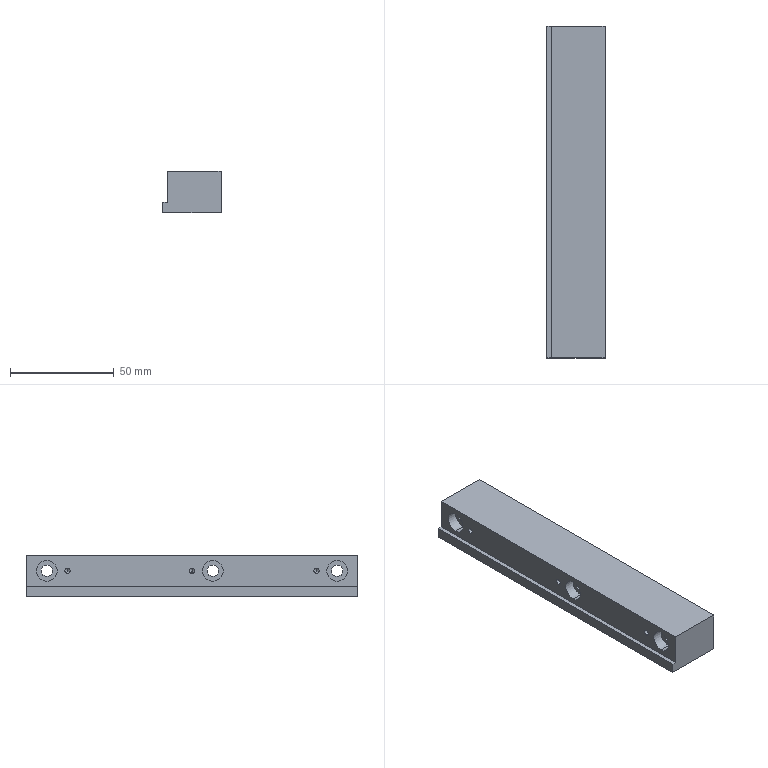Part | SolidWorks | features LPattern 3, HoleWzd 2, Extrusion 1, ICE 1 | 1 solid | 35 faces | box 28 x 160 x 20 mm | volume 82011 mm3 | cylinder 18 | plane 11 | cone 6 | commonest cylinder face diameters 2.5 x6 5.5 x6 10 x6
STEP:
#1=CARTESIAN_POINT('',(7.,-10.,-2.5));
#2=VERTEX_POINT('',#1);
#3=CARTESIAN_POINT('',(7.,-10.,7.5));
#4=VERTEX_POINT('',#3);
#5=CARTESIAN_POINT('',(7.,-10.,2.5));
#6=DIRECTION('',(-1.,0.,0.));
#7=DIRECTION('',(0.,0.,1.));
#8=AXIS2_PLACEMENT_3D('',#5,#6,#7);
#9=CIRCLE('',#8,5.);
#10=EDGE_CURVE('',#2,#4,#9,.T.);
#11=ORIENTED_EDGE('',*,*,#10,.F.);
#12=CARTESIAN_POINT('',(2.,-10.,-2.5));
#13=VERTEX_POINT('',#12);
#14=CARTESIAN_POINT('',(2.,-10.,-2.5));
#15=DIRECTION('',(-1.,0.,0.));
#16=VECTOR('',#15,1000.);
#17=LINE('',#14,#16);
#18=EDGE_CURVE('',#2,#13,#17,.T.);
#19=ORIENTED_EDGE('',*,*,#18,.T.);
#20=CARTESIAN_POINT('',(2.,-10.,7.5));
#21=VERTEX_POINT('',#20);
#22=CARTESIAN_POINT('',(2.,-10.,2.5));
#23=DIRECTION('',(-1.,0.,0.));
#24=DIRECTION('',(0.,0.,1.));
#25=AXIS2_PLACEMENT_3D('',#22,#23,#24);
#26=CIRCLE('',#25,5.);
#27=EDGE_CURVE('',#13,#21,#26,.T.);
#28=ORIENTED_EDGE('',*,*,#27,.T.);
#29=CARTESIAN_POINT('',(2.,-10.,7.5));
#30=DIRECTION('',(-1.,0.,0.));
#31=VECTOR('',#30,1000.);
#32=LINE('',#29,#31);
#33=EDGE_CURVE('',#4,#21,#32,.T.);
#34=ORIENTED_EDGE('',*,*,#33,.F.);
#35=EDGE_LOOP('',(#11,#19,#28,#34));
#36=FACE_OUTER_BOUND('',#35,.T.);
#37=CARTESIAN_POINT('',(2.,-10.,2.5));
#38=DIRECTION('',(-1.,0.,0.));
#39=DIRECTION('',(0.,0.,1.));
#40=AXIS2_PLACEMENT_3D('',#37,#38,#39);
#41=CYLINDRICAL_SURFACE('',#40,5.);
#42=ADVANCED_FACE('',(#36),#41,.F.);
#43=CARTESIAN_POINT('',(28.,-10.,-0.25));
#44=VERTEX_POINT('',#43);
#45=CARTESIAN_POINT('',(28.,-10.,5.25));
#46=VERTEX_POINT('',#45);
#47=CARTESIAN_POINT('',(28.,-10.,2.5));
#48=DIRECTION('',(-1.,0.,0.));
#49=DIRECTION('',(0.,0.,1.));
#50=AXIS2_PLACEMENT_3D('',#47,#48,#49);
#51=CIRCLE('',#50,2.75);
#52=EDGE_CURVE('',#44,#46,#51,.T.);
#53=ORIENTED_EDGE('',*,*,#52,.F.);
#54=CARTESIAN_POINT('',(7.,-10.,-0.25));
#55=VERTEX_POINT('',#54);
#56=CARTESIAN_POINT('',(2.,-10.,-0.25));
#57=DIRECTION('',(-1.,0.,0.));
#58=VECTOR('',#57,1000.);
#59=LINE('',#56,#58);
#60=EDGE_CURVE('',#44,#55,#59,.T.);
#61=ORIENTED_EDGE('',*,*,#60,.T.);
#62=CARTESIAN_POINT('',(7.,-10.,5.25));
#63=VERTEX_POINT('',#62);
#64=CARTESIAN_POINT('',(7.,-10.,2.5));
#65=DIRECTION('',(-1.,0.,0.));
#66=DIRECTION('',(0.,0.,1.));
#67=AXIS2_PLACEMENT_3D('',#64,#65,#66);
#68=CIRCLE('',#67,2.75);
#69=EDGE_CURVE('',#55,#63,#68,.T.);
#70=ORIENTED_EDGE('',*,*,#69,.T.);
#71=CARTESIAN_POINT('',(2.,-10.,5.25));
#72=DIRECTION('',(-1.,0.,0.));
#73=VECTOR('',#72,1000.);
#74=LINE('',#71,#73);
#75=EDGE_CURVE('',#46,#63,#74,.T.);
#76=ORIENTED_EDGE('',*,*,#75,.F.);
#77=EDGE_LOOP('',(#53,#61,#70,#76));
#78=FACE_OUTER_BOUND('',#77,.T.);
#79=CARTESIAN_POINT('',(2.,-10.,2.5));
#80=DIRECTION('',(-1.,0.,0.));
#81=DIRECTION('',(0.,0.,1.));
#82=AXIS2_PLACEMENT_3D('',#79,#80,#81);
#83=CYLINDRICAL_SURFACE('',#82,2.75);
#84=ADVANCED_FACE('',(#78),#83,.F.);
#85=CARTESIAN_POINT('',(7.,70.,-2.5));
#86=VERTEX_POINT('',#85);
#87=CARTESIAN_POINT('',(7.,70.,7.5));
#88=VERTEX_POINT('',#87);
#89=CARTESIAN_POINT('',(7.,70.,2.5));
#90=DIRECTION('',(-1.,0.,0.));
#91=DIRECTION('',(0.,0.,1.));
#92=AXIS2_PLACEMENT_3D('',#89,#90,#91);
#93=CIRCLE('',#92,5.);
#94=EDGE_CURVE('',#86,#88,#93,.T.);
#95=ORIENTED_EDGE('',*,*,#94,.F.);
#96=CARTESIAN_POINT('',(2.,70.,-2.5));
#97=VERTEX_POINT('',#96);
#98=CARTESIAN_POINT('',(2.,70.,-2.5));
#99=DIRECTION('',(-1.,0.,0.));
#100=VECTOR('',#99,1000.);
#101=LINE('',#98,#100);
#102=EDGE_CURVE('',#86,#97,#101,.T.);
#103=ORIENTED_EDGE('',*,*,#102,.T.);
#104=CARTESIAN_POINT('',(2.,70.,7.5));
#105=VERTEX_POINT('',#104);
#106=CARTESIAN_POINT('',(2.,70.,2.5));
#107=DIRECTION('',(-1.,0.,0.));
#108=DIRECTION('',(0.,0.,1.));
#109=AXIS2_PLACEMENT_3D('',#106,#107,#108);
#110=CIRCLE('',#109,5.);
#111=EDGE_CURVE('',#97,#105,#110,.T.);
#112=ORIENTED_EDGE('',*,*,#111,.T.);
#113=CARTESIAN_POINT('',(2.,70.,7.5));
#114=DIRECTION('',(-1.,0.,0.));
#115=VECTOR('',#114,1000.);
#116=LINE('',#113,#115);
#117=EDGE_CURVE('',#88,#105,#116,.T.);
#118=ORIENTED_EDGE('',*,*,#117,.F.);
#119=EDGE_LOOP('',(#95,#103,#112,#118));
#120=FACE_OUTER_BOUND('',#119,.T.);
#121=CARTESIAN_POINT('',(2.,70.,2.5));
#122=DIRECTION('',(-1.,0.,0.));
#123=DIRECTION('',(0.,0.,1.));
#124=AXIS2_PLACEMENT_3D('',#121,#122,#123);
#125=CYLINDRICAL_SURFACE('',#124,5.);
#126=ADVANCED_FACE('',(#120),#125,.F.);
#127=CARTESIAN_POINT('',(28.,70.,-0.25));
#128=VERTEX_POINT('',#127);
#129=CARTESIAN_POINT('',(28.,70.,5.25));
#130=VERTEX_POINT('',#129);
#131=CARTESIAN_POINT('',(28.,70.,2.5));
#132=DIRECTION('',(-1.,0.,0.));
#133=DIRECTION('',(0.,0.,1.));
#134=AXIS2_PLACEMENT_3D('',#131,#132,#133);
#135=CIRCLE('',#134,2.75);
#136=EDGE_CURVE('',#128,#130,#135,.T.);
#137=ORIENTED_EDGE('',*,*,#136,.F.);
#138=CARTESIAN_POINT('',(7.,70.,-0.25));
#139=VERTEX_POINT('',#138);
#140=CARTESIAN_POINT('',(2.,70.,-0.25));
#141=DIRECTION('',(-1.,0.,0.));
#142=VECTOR('',#141,1000.);
#143=LINE('',#140,#142);
#144=EDGE_CURVE('',#128,#139,#143,.T.);
#145=ORIENTED_EDGE('',*,*,#144,.T.);
#146=CARTESIAN_POINT('',(7.,70.,5.25));
#147=VERTEX_POINT('',#146);
#148=CARTESIAN_POINT('',(7.,70.,2.5));
#149=DIRECTION('',(-1.,0.,0.));
#150=DIRECTION('',(0.,0.,1.));
#151=AXIS2_PLACEMENT_3D('',#148,#149,#150);
#152=CIRCLE('',#151,2.75);
#153=EDGE_CURVE('',#139,#147,#152,.T.);
#154=ORIENTED_EDGE('',*,*,#153,.T.);
#155=CARTESIAN_POINT('',(2.,70.,5.25));
#156=DIRECTION('',(-1.,0.,0.));
#157=VECTOR('',#156,1000.);
#158=LINE('',#155,#157);
#159=EDGE_CURVE('',#130,#147,#158,.T.);
#160=ORIENTED_EDGE('',*,*,#159,.F.);
#161=EDGE_LOOP('',(#137,#145,#154,#160));
#162=FACE_OUTER_BOUND('',#161,.T.);
#163=CARTESIAN_POINT('',(2.,70.,2.5));
#164=DIRECTION('',(-1.,0.,0.));
#165=DIRECTION('',(0.,0.,1.));
#166=AXIS2_PLACEMENT_3D('',#163,#164,#165);
#167=CYLINDRICAL_SURFACE('',#166,2.75);
#168=ADVANCED_FACE('',(#162),#167,.F.);
#169=CARTESIAN_POINT('',(7.,-70.,-2.5));
#170=VERTEX_POINT('',#169);
#171=CARTESIAN_POINT('',(7.,-70.,7.5));
#172=VERTEX_POINT('',#171);
#173=CARTESIAN_POINT('',(7.,-70.,2.5));
#174=DIRECTION('',(-1.,0.,0.));
#175=DIRECTION('',(0.,0.,1.));
#176=AXIS2_PLACEMENT_3D('',#173,#174,#175);
#177=CIRCLE('',#176,5.);
#178=EDGE_CURVE('',#170,#172,#177,.T.);
#179=ORIENTED_EDGE('',*,*,#178,.F.);
#180=CARTESIAN_POINT('',(2.,-70.,-2.5));
#181=VERTEX_POINT('',#180);
#182=CARTESIAN_POINT('',(2.,-70.,-2.5));
#183=DIRECTION('',(-1.,0.,0.));
#184=VECTOR('',#183,1000.);
#185=LINE('',#182,#184);
#186=EDGE_CURVE('',#170,#181,#185,.T.);
#187=ORIENTED_EDGE('',*,*,#186,.T.);
#188=CARTESIAN_POINT('',(2.,-70.,7.5));
#189=VERTEX_POINT('',#188);
#190=CARTESIAN_POINT('',(2.,-70.,2.5));
#191=DIRECTION('',(-1.,0.,0.));
#192=DIRECTION('',(0.,0.,1.));
#193=AXIS2_PLACEMENT_3D('',#190,#191,#192);
#194=CIRCLE('',#193,5.);
#195=EDGE_CURVE('',#181,#189,#194,.T.);
#196=ORIENTED_EDGE('',*,*,#195,.T.);
#197=CARTESIAN_POINT('',(2.,-70.,7.5));
#198=DIRECTION('',(-1.,0.,0.));
#199=VECTOR('',#198,1000.);
#200=LINE('',#197,#199);
#201=EDGE_CURVE('',#172,#189,#200,.T.);
#202=ORIENTED_EDGE('',*,*,#201,.F.);
#203=EDGE_LOOP('',(#179,#187,#196,#202));
#204=FACE_OUTER_BOUND('',#203,.T.);
#205=CARTESIAN_POINT('',(2.,-70.,2.5));
#206=DIRECTION('',(-1.,0.,0.));
#207=DIRECTION('',(0.,0.,1.));
#208=AXIS2_PLACEMENT_3D('',#205,#206,#207);
#209=CYLINDRICAL_SURFACE('',#208,5.);
#210=ADVANCED_FACE('',(#204),#209,.F.);
#211=CARTESIAN_POINT('',(28.,-70.,-0.25));
#212=VERTEX_POINT('',#211);
#213=CARTESIAN_POINT('',(28.,-70.,5.25));
#214=VERTEX_POINT('',#213);
#215=CARTESIAN_POINT('',(28.,-70.,2.5));
#216=DIRECTION('',(-1.,0.,0.));
#217=DIRECTION('',(0.,0.,1.));
#218=AXIS2_PLACEMENT_3D('',#215,#216,#217);
#219=CIRCLE('',#218,2.75);
#220=EDGE_CURVE('',#212,#214,#219,.T.);
#221=ORIENTED_EDGE('',*,*,#220,.F.);
#222=CARTESIAN_POINT('',(7.,-70.,-0.25));
#223=VERTEX_POINT('',#222);
#224=CARTESIAN_POINT('',(2.,-70.,-0.25));
#225=DIRECTION('',(-1.,0.,0.));
#226=VECTOR('',#225,1000.);
#227=LINE('',#224,#226);
#228=EDGE_CURVE('',#212,#223,#227,.T.);
#229=ORIENTED_EDGE('',*,*,#228,.T.);
#230=CARTESIAN_POINT('',(7.,-70.,5.25));
#231=VERTEX_POINT('',#230);
#232=CARTESIAN_POINT('',(7.,-70.,2.5));
#233=DIRECTION('',(-1.,0.,0.));
#234=DIRECTION('',(0.,0.,1.));
#235=AXIS2_PLACEMENT_3D('',#232,#233,#234);
#236=CIRCLE('',#235,2.75);
#237=EDGE_CURVE('',#223,#231,#236,.T.);
#238=ORIENTED_EDGE('',*,*,#237,.T.);
#239=CARTESIAN_POINT('',(2.,-70.,5.25));
#240=DIRECTION('',(-1.,0.,0.));
#241=VECTOR('',#240,1000.);
#242=LINE('',#239,#241);
#243=EDGE_CURVE('',#214,#231,#242,.T.);
#244=ORIENTED_EDGE('',*,*,#243,.F.);
#245=EDGE_LOOP('',(#221,#229,#238,#244));
#246=FACE_OUTER_BOUND('',#245,.T.);
#247=CARTESIAN_POINT('',(2.,-70.,2.5));
#248=DIRECTION('',(-1.,0.,0.));
#249=DIRECTION('',(0.,0.,1.));
#250=AXIS2_PLACEMENT_3D('',#247,#248,#249);
#251=CYLINDRICAL_SURFACE('',#250,2.75);
#252=ADVANCED_FACE('',(#246),#251,.F.);
#253=CARTESIAN_POINT('',(10.251,60.,2.5));
#254=VERTEX_POINT('',#253);
#255=CARTESIAN_POINT('',(9.5,60.,3.75));
#256=VERTEX_POINT('',#255);
#257=CARTESIAN_POINT('',(9.5,60.,3.75));
#258=DIRECTION('',(-0.515,0.,0.8572));
#259=VECTOR('',#258,1000.);
#260=LINE('',#257,#259);
#261=EDGE_CURVE('',#254,#256,#260,.T.);
#262=ORIENTED_EDGE('',*,*,#261,.F.);
#263=CARTESIAN_POINT('',(9.5,60.,1.25));
#264=VERTEX_POINT('',#263);
#265=CARTESIAN_POINT('',(9.5,60.,1.25));
#266=DIRECTION('',(-0.515,0.,-0.8572));
#267=VECTOR('',#266,1000.);
#268=LINE('',#265,#267);
#269=EDGE_CURVE('',#254,#264,#268,.T.);
#270=ORIENTED_EDGE('',*,*,#269,.T.);
#271=CARTESIAN_POINT('',(9.5,60.,2.5));
#272=DIRECTION('',(-1.,0.,0.));
#273=DIRECTION('',(0.,0.,1.));
#274=AXIS2_PLACEMENT_3D('',#271,#272,#273);
#275=CIRCLE('',#274,1.25);
#276=EDGE_CURVE('',#264,#256,#275,.T.);
#277=ORIENTED_EDGE('',*,*,#276,.T.);
#278=EDGE_LOOP('',(#262,#270,#277));
#279=FACE_OUTER_BOUND('',#278,.T.);
#280=CARTESIAN_POINT('',(9.5,60.,2.5));
#281=DIRECTION('',(-1.,0.,0.));
#282=DIRECTION('',(0.,0.,1.));
#283=AXIS2_PLACEMENT_3D('',#280,#281,#282);
#284=CONICAL_SURFACE('',#283,1.25,1.03);
#285=ADVANCED_FACE('',(#279),#284,.F.);
#286=ORIENTED_EDGE('',*,*,#276,.F.);
#287=CARTESIAN_POINT('',(2.,60.,1.25));
#288=VERTEX_POINT('',#287);
#289=CARTESIAN_POINT('',(2.,60.,1.25));
#290=DIRECTION('',(-1.,0.,0.));
#291=VECTOR('',#290,1000.);
#292=LINE('',#289,#291);
#293=EDGE_CURVE('',#264,#288,#292,.T.);
#294=ORIENTED_EDGE('',*,*,#293,.T.);
#295=CARTESIAN_POINT('',(2.,60.,3.75));
#296=VERTEX_POINT('',#295);
#297=CARTESIAN_POINT('',(2.,60.,2.5));
#298=DIRECTION('',(-1.,0.,0.));
#299=DIRECTION('',(0.,0.,1.));
#300=AXIS2_PLACEMENT_3D('',#297,#298,#299);
#301=CIRCLE('',#300,1.25);
#302=EDGE_CURVE('',#288,#296,#301,.T.);
#303=ORIENTED_EDGE('',*,*,#302,.T.);
#304=CARTESIAN_POINT('',(2.,60.,3.75));
#305=DIRECTION('',(-1.,0.,0.));
#306=VECTOR('',#305,1000.);
#307=LINE('',#304,#306);
#308=EDGE_CURVE('',#256,#296,#307,.T.);
#309=ORIENTED_EDGE('',*,*,#308,.F.);
#310=EDGE_LOOP('',(#286,#294,#303,#309));
#311=FACE_OUTER_BOUND('',#310,.T.);
#312=CARTESIAN_POINT('',(2.,60.,2.5));
#313=DIRECTION('',(-1.,0.,0.));
#314=DIRECTION('',(0.,0.,1.));
#315=AXIS2_PLACEMENT_3D('',#312,#313,#314);
#316=CYLINDRICAL_SURFACE('',#315,1.25);
#317=ADVANCED_FACE('',(#311),#316,.F.);
#318=CARTESIAN_POINT('',(9.5,0.,1.25));
#319=VERTEX_POINT('',#318);
#320=CARTESIAN_POINT('',(9.5,0.,3.75));
#321=VERTEX_POINT('',#320);
#322=CARTESIAN_POINT('',(9.5,0.,2.5));
#323=DIRECTION('',(-1.,0.,0.));
#324=DIRECTION('',(0.,0.,1.));
#325=AXIS2_PLACEMENT_3D('',#322,#323,#324);
#326=CIRCLE('',#325,1.25);
#327=EDGE_CURVE('',#319,#321,#326,.T.);
#328=ORIENTED_EDGE('',*,*,#327,.F.);
#329=CARTESIAN_POINT('',(2.,0.,1.25));
#330=VERTEX_POINT('',#329);
#331=CARTESIAN_POINT('',(2.,0.,1.25));
#332=DIRECTION('',(-1.,0.,0.));
#333=VECTOR('',#332,1000.);
#334=LINE('',#331,#333);
#335=EDGE_CURVE('',#319,#330,#334,.T.);
#336=ORIENTED_EDGE('',*,*,#335,.T.);
#337=CARTESIAN_POINT('',(2.,0.,3.75));
#338=VERTEX_POINT('',#337);
#339=CARTESIAN_POINT('',(2.,0.,2.5));
#340=DIRECTION('',(-1.,0.,0.));
#341=DIRECTION('',(0.,0.,1.));
#342=AXIS2_PLACEMENT_3D('',#339,#340,#341);
#343=CIRCLE('',#342,1.25);
#344=EDGE_CURVE('',#330,#338,#343,.T.);
#345=ORIENTED_EDGE('',*,*,#344,.T.);
#346=CARTESIAN_POINT('',(2.,0.,3.75));
#347=DIRECTION('',(-1.,0.,0.));
#348=VECTOR('',#347,1000.);
#349=LINE('',#346,#348);
#350=EDGE_CURVE('',#321,#338,#349,.T.);
#351=ORIENTED_EDGE('',*,*,#350,.F.);
#352=EDGE_LOOP('',(#328,#336,#345,#351));
#353=FACE_OUTER_BOUND('',#352,.T.);
#354=CARTESIAN_POINT('',(2.,0.,2.5));
#355=DIRECTION('',(-1.,0.,0.));
#356=DIRECTION('',(0.,0.,1.));
#357=AXIS2_PLACEMENT_3D('',#354,#355,#356);
#358=CYLINDRICAL_SURFACE('',#357,1.25);
#359=ADVANCED_FACE('',(#353),#358,.F.);
#360=CARTESIAN_POINT('',(10.251,0.,2.5));
#361=VERTEX_POINT('',#360);
#362=CARTESIAN_POINT('',(9.5,0.,3.75));
#363=DIRECTION('',(-0.515,0.,0.8572));
#364=VECTOR('',#363,1000.);
#365=LINE('',#362,#364);
#366=EDGE_CURVE('',#361,#321,#365,.T.);
#367=ORIENTED_EDGE('',*,*,#366,.F.);
#368=CARTESIAN_POINT('',(9.5,0.,1.25));
#369=DIRECTION('',(-0.515,0.,-0.8572));
#370=VECTOR('',#369,1000.);
#371=LINE('',#368,#370);
#372=EDGE_CURVE('',#361,#319,#371,.T.);
#373=ORIENTED_EDGE('',*,*,#372,.T.);
#374=ORIENTED_EDGE('',*,*,#327,.T.);
#375=EDGE_LOOP('',(#367,#373,#374));
#376=FACE_OUTER_BOUND('',#375,.T.);
#377=CARTESIAN_POINT('',(9.5,0.,2.5));
#378=DIRECTION('',(-1.,0.,0.));
#379=DIRECTION('',(0.,0.,1.));
#380=AXIS2_PLACEMENT_3D('',#377,#378,#379);
#381=CONICAL_SURFACE('',#380,1.25,1.03);
#382=ADVANCED_FACE('',(#376),#381,.F.);
#383=CARTESIAN_POINT('',(9.5,-60.,1.25));
#384=VERTEX_POINT('',#383);
#385=CARTESIAN_POINT('',(9.5,-60.,3.75));
#386=VERTEX_POINT('',#385);
#387=CARTESIAN_POINT('',(9.5,-60.,2.5));
#388=DIRECTION('',(-1.,0.,0.));
#389=DIRECTION('',(0.,0.,1.));
#390=AXIS2_PLACEMENT_3D('',#387,#388,#389);
#391=CIRCLE('',#390,1.25);
#392=EDGE_CURVE('',#384,#386,#391,.T.);
#393=ORIENTED_EDGE('',*,*,#392,.F.);
#394=CARTESIAN_POINT('',(2.,-60.,1.25));
#395=VERTEX_POINT('',#394);
#396=CARTESIAN_POINT('',(2.,-60.,1.25));
#397=DIRECTION('',(-1.,0.,0.));
#398=VECTOR('',#397,1000.);
#399=LINE('',#396,#398);
#400=EDGE_CURVE('',#384,#395,#399,.T.);
#401=ORIENTED_EDGE('',*,*,#400,.T.);
#402=CARTESIAN_POINT('',(2.,-60.,3.75));
#403=VERTEX_POINT('',#402);
#404=CARTESIAN_POINT('',(2.,-60.,2.5));
#405=DIRECTION('',(-1.,0.,0.));
#406=DIRECTION('',(0.,0.,1.));
#407=AXIS2_PLACEMENT_3D('',#404,#405,#406);
#408=CIRCLE('',#407,1.25);
#409=EDGE_CURVE('',#395,#403,#408,.T.);
#410=ORIENTED_EDGE('',*,*,#409,.T.);
#411=CARTESIAN_POINT('',(2.,-60.,3.75));
#412=DIRECTION('',(-1.,0.,0.));
#413=VECTOR('',#412,1000.);
#414=LINE('',#411,#413);
#415=EDGE_CURVE('',#386,#403,#414,.T.);
#416=ORIENTED_EDGE('',*,*,#415,.F.);
#417=EDGE_LOOP('',(#393,#401,#410,#416));
#418=FACE_OUTER_BOUND('',#417,.T.);
#419=CARTESIAN_POINT('',(2.,-60.,2.5));
#420=DIRECTION('',(-1.,0.,0.));
#421=DIRECTION('',(0.,0.,1.));
#422=AXIS2_PLACEMENT_3D('',#419,#420,#421);
#423=CYLINDRICAL_SURFACE('',#422,1.25);
#424=ADVANCED_FACE('',(#418),#423,.F.);
#425=CARTESIAN_POINT('',(10.251,-60.,2.5));
#426=VERTEX_POINT('',#425);
#427=CARTESIAN_POINT('',(9.5,-60.,3.75));
#428=DIRECTION('',(-0.515,0.,0.8572));
#429=VECTOR('',#428,1000.);
#430=LINE('',#427,#429);
#431=EDGE_CURVE('',#426,#386,#430,.T.);
#432=ORIENTED_EDGE('',*,*,#431,.F.);
#433=CARTESIAN_POINT('',(9.5,-60.,1.25));
#434=DIRECTION('',(-0.515,0.,-0.8572));
#435=VECTOR('',#434,1000.);
#436=LINE('',#433,#435);
#437=EDGE_CURVE('',#426,#384,#436,.T.);
#438=ORIENTED_EDGE('',*,*,#437,.T.);
#439=ORIENTED_EDGE('',*,*,#392,.T.);
#440=EDGE_LOOP('',(#432,#438,#439));
#441=FACE_OUTER_BOUND('',#440,.T.);
#442=CARTESIAN_POINT('',(9.5,-60.,2.5));
#443=DIRECTION('',(-1.,0.,0.));
#444=DIRECTION('',(0.,0.,1.));
#445=AXIS2_PLACEMENT_3D('',#442,#443,#444);
#446=CONICAL_SURFACE('',#445,1.25,1.03);
#447=ADVANCED_FACE('',(#441),#446,.F.);
#448=CARTESIAN_POINT('',(2.,-10.,2.5));
#449=DIRECTION('',(-1.,0.,0.));
#450=DIRECTION('',(0.,0.,1.));
#451=AXIS2_PLACEMENT_3D('',#448,#449,#450);
#452=CIRCLE('',#451,5.);
#453=EDGE_CURVE('',#21,#13,#452,.T.);
#454=ORIENTED_EDGE('',*,*,#453,.F.);
#455=ORIENTED_EDGE('',*,*,#27,.F.);
#456=EDGE_LOOP('',(#454,#455));
#457=FACE_BOUND('',#456,.T.);
#458=CARTESIAN_POINT('',(2.,70.,2.5));
#459=DIRECTION('',(-1.,0.,0.));
#460=DIRECTION('',(0.,0.,1.));
#461=AXIS2_PLACEMENT_3D('',#458,#459,#460);
#462=CIRCLE('',#461,5.);
#463=EDGE_CURVE('',#105,#97,#462,.T.);
#464=ORIENTED_EDGE('',*,*,#463,.F.);
#465=ORIENTED_EDGE('',*,*,#111,.F.);
#466=EDGE_LOOP('',(#464,#465));
#467=FACE_BOUND('',#466,.T.);
#468=CARTESIAN_POINT('',(2.,60.,2.5));
#469=DIRECTION('',(-1.,0.,0.));
#470=DIRECTION('',(0.,0.,1.));
#471=AXIS2_PLACEMENT_3D('',#468,#469,#470);
#472=CIRCLE('',#471,1.25);
#473=EDGE_CURVE('',#296,#288,#472,.T.);
#474=ORIENTED_EDGE('',*,*,#473,.F.);
#475=ORIENTED_EDGE('',*,*,#302,.F.);
#476=EDGE_LOOP('',(#474,#475));
#477=FACE_BOUND('',#476,.T.);
#478=CARTESIAN_POINT('',(2.,-80.,10.));
#479=VERTEX_POINT('',#478);
#480=CARTESIAN_POINT('',(2.,80.,10.));
#481=VERTEX_POINT('',#480);
#482=CARTESIAN_POINT('',(2.,80.,10.));
#483=DIRECTION('',(0.,1.,0.));
#484=VECTOR('',#483,1000.);
#485=LINE('',#482,#484);
#486=EDGE_CURVE('',#479,#481,#485,.T.);
#487=ORIENTED_EDGE('',*,*,#486,.T.);
#488=CARTESIAN_POINT('',(2.,80.,-5.));
#489=VERTEX_POINT('',#488);
#490=CARTESIAN_POINT('',(2.,80.,10.));
#491=DIRECTION('',(0.,0.,-1.));
#492=VECTOR('',#491,1000.);
#493=LINE('',#490,#492);
#494=EDGE_CURVE('',#481,#489,#493,.T.);
#495=ORIENTED_EDGE('',*,*,#494,.T.);
#496=CARTESIAN_POINT('',(2.,-80.,-5.));
#497=VERTEX_POINT('',#496);
#498=CARTESIAN_POINT('',(2.,80.,-5.));
#499=DIRECTION('',(0.,-1.,0.));
#500=VECTOR('',#499,1000.);
#501=LINE('',#498,#500);
#502=EDGE_CURVE('',#489,#497,#501,.T.);
#503=ORIENTED_EDGE('',*,*,#502,.T.);
#504=CARTESIAN_POINT('',(2.,-80.,10.));
#505=DIRECTION('',(0.,0.,1.));
#506=VECTOR('',#505,1000.);
#507=LINE('',#504,#506);
#508=EDGE_CURVE('',#497,#479,#507,.T.);
#509=ORIENTED_EDGE('',*,*,#508,.T.);
#510=EDGE_LOOP('',(#487,#495,#503,#509));
#511=FACE_OUTER_BOUND('',#510,.T.);
#512=CARTESIAN_POINT('',(2.,-60.,2.5));
#513=DIRECTION('',(-1.,0.,0.));
#514=DIRECTION('',(0.,0.,1.));
#515=AXIS2_PLACEMENT_3D('',#512,#513,#514);
#516=CIRCLE('',#515,1.25);
#517=EDGE_CURVE('',#403,#395,#516,.T.);
#518=ORIENTED_EDGE('',*,*,#517,.F.);
#519=ORIENTED_EDGE('',*,*,#409,.F.);
#520=EDGE_LOOP('',(#518,#519));
#521=FACE_BOUND('',#520,.T.);
#522=CARTESIAN_POINT('',(2.,0.,2.5));
#523=DIRECTION('',(-1.,0.,0.));
#524=DIRECTION('',(0.,0.,1.));
#525=AXIS2_PLACEMENT_3D('',#522,#523,#524);
#526=CIRCLE('',#525,1.25);
#527=EDGE_CURVE('',#338,#330,#526,.T.);
#528=ORIENTED_EDGE('',*,*,#527,.F.);
#529=ORIENTED_EDGE('',*,*,#344,.F.);
#530=EDGE_LOOP('',(#528,#529));
#531=FACE_BOUND('',#530,.T.);
#532=CARTESIAN_POINT('',(2.,-70.,2.5));
#533=DIRECTION('',(-1.,0.,0.));
#534=DIRECTION('',(0.,0.,1.));
#535=AXIS2_PLACEMENT_3D('',#532,#533,#534);
#536=CIRCLE('',#535,5.);
#537=EDGE_CURVE('',#189,#181,#536,.T.);
#538=ORIENTED_EDGE('',*,*,#537,.F.);
#539=ORIENTED_EDGE('',*,*,#195,.F.);
#540=EDGE_LOOP('',(#538,#539));
#541=FACE_BOUND('',#540,.T.);
#542=CARTESIAN_POINT('',(2.,-80.,10.));
#543=DIRECTION('',(1.,0.,0.));
#544=DIRECTION('',(0.,0.,-1.));
#545=AXIS2_PLACEMENT_3D('',#542,#543,#544);
#546=PLANE('',#545);
#547=ADVANCED_FACE('',(#457,#467,#477,#511,#521,#531,#541),#546,.F.);
#548=CARTESIAN_POINT('',(0.,-80.,-10.));
#549=VERTEX_POINT('',#548);
#550=CARTESIAN_POINT('',(0.,80.,-10.));
#551=VERTEX_POINT('',#550);
#552=CARTESIAN_POINT('',(0.,-80.,-10.));
#553=DIRECTION('',(0.,1.,0.));
#554=VECTOR('',#553,1000.);
#555=LINE('',#552,#554);
#556=EDGE_CURVE('',#549,#551,#555,.T.);
#557=ORIENTED_EDGE('',*,*,#556,.T.);
#558=CARTESIAN_POINT('',(28.,80.,-10.));
#559=VERTEX_POINT('',#558);
#560=CARTESIAN_POINT('',(28.,80.,-10.));
#561=DIRECTION('',(-1.,0.,0.));
#562=VECTOR('',#561,1000.);
#563=LINE('',#560,#562);
#564=EDGE_CURVE('',#559,#551,#563,.T.);
#565=ORIENTED_EDGE('',*,*,#564,.F.);
#566=CARTESIAN_POINT('',(28.,-80.,-10.));
#567=VERTEX_POINT('',#566);
#568=CARTESIAN_POINT('',(28.,-80.,-10.));
#569=DIRECTION('',(0.,1.,0.));
#570=VECTOR('',#569,1000.);
#571=LINE('',#568,#570);
#572=EDGE_CURVE('',#567,#559,#571,.T.);
#573=ORIENTED_EDGE('',*,*,#572,.F.);
#574=CARTESIAN_POINT('',(28.,-80.,-10.));
#575=DIRECTION('',(-1.,0.,0.));
#576=VECTOR('',#575,1000.);
#577=LINE('',#574,#576);
#578=EDGE_CURVE('',#567,#549,#577,.T.);
#579=ORIENTED_EDGE('',*,*,#578,.T.);
#580=EDGE_LOOP('',(#557,#565,#573,#579));
#581=FACE_OUTER_BOUND('',#580,.T.);
#582=CARTESIAN_POINT('',(28.,-80.,-10.));
#583=DIRECTION('',(0.,0.,1.));
#584=DIRECTION('',(1.,0.,0.));
#585=AXIS2_PLACEMENT_3D('',#582,#583,#584);
#586=PLANE('',#585);
#587=ADVANCED_FACE('',(#581),#586,.F.);
#588=CARTESIAN_POINT('',(0.,80.,-5.));
#589=VERTEX_POINT('',#588);
#590=CARTESIAN_POINT('',(0.,80.,10.));
#591=DIRECTION('',(0.,0.,1.));
#592=VECTOR('',#591,1000.);
#593=LINE('',#590,#592);
#594=EDGE_CURVE('',#551,#589,#593,.T.);
#595=ORIENTED_EDGE('',*,*,#594,.T.);
#596=CARTESIAN_POINT('',(2.,80.,-5.));
#597=DIRECTION('',(-1.,0.,0.));
#598=VECTOR('',#597,1000.);
#599=LINE('',#596,#598);
#600=EDGE_CURVE('',#489,#589,#599,.T.);
#601=ORIENTED_EDGE('',*,*,#600,.F.);
#602=ORIENTED_EDGE('',*,*,#494,.F.);
#603=CARTESIAN_POINT('',(28.,80.,10.));
#604=VERTEX_POINT('',#603);
#605=CARTESIAN_POINT('',(28.,80.,10.));
#606=DIRECTION('',(-1.,0.,0.));
#607=VECTOR('',#606,1000.);
#608=LINE('',#605,#607);
#609=EDGE_CURVE('',#604,#481,#608,.T.);
#610=ORIENTED_EDGE('',*,*,#609,.F.);
#611=CARTESIAN_POINT('',(28.,80.,10.));
#612=DIRECTION('',(0.,0.,1.));
#613=VECTOR('',#612,1000.);
#614=LINE('',#611,#613);
#615=EDGE_CURVE('',#559,#604,#614,.T.);
#616=ORIENTED_EDGE('',*,*,#615,.F.);
#617=ORIENTED_EDGE('',*,*,#564,.T.);
#618=EDGE_LOOP('',(#595,#601,#602,#610,#616,#617));
#619=FACE_OUTER_BOUND('',#618,.T.);
#620=CARTESIAN_POINT('',(28.,80.,10.));
#621=DIRECTION('',(0.,-1.,0.));
#622=DIRECTION('',(0.,0.,-1.));
#623=AXIS2_PLACEMENT_3D('',#620,#621,#622);
#624=PLANE('',#623);
#625=ADVANCED_FACE('',(#619),#624,.F.);
#626=ORIENTED_EDGE('',*,*,#609,.T.);
#627=ORIENTED_EDGE('',*,*,#486,.F.);
#628=CARTESIAN_POINT('',(28.,-80.,10.));
#629=VERTEX_POINT('',#628);
#630=CARTESIAN_POINT('',(28.,-80.,10.));
#631=DIRECTION('',(-1.,0.,0.));
#632=VECTOR('',#631,1000.);
#633=LINE('',#630,#632);
#634=EDGE_CURVE('',#629,#479,#633,.T.);
#635=ORIENTED_EDGE('',*,*,#634,.F.);
#636=CARTESIAN_POINT('',(28.,-80.,10.));
#637=DIRECTION('',(0.,-1.,0.));
#638=VECTOR('',#637,1000.);
#639=LINE('',#636,#638);
#640=EDGE_CURVE('',#604,#629,#639,.T.);
#641=ORIENTED_EDGE('',*,*,#640,.F.);
#642=EDGE_LOOP('',(#626,#627,#635,#641));
#643=FACE_OUTER_BOUND('',#642,.T.);
#644=CARTESIAN_POINT('',(28.,-80.,10.));
#645=DIRECTION('',(0.,0.,-1.));
#646=DIRECTION('',(-1.,0.,0.));
#647=AXIS2_PLACEMENT_3D('',#644,#645,#646);
#648=PLANE('',#647);
#649=ADVANCED_FACE('',(#643),#648,.F.);
#650=ORIENTED_EDGE('',*,*,#508,.F.);
#651=CARTESIAN_POINT('',(0.,-80.,-5.));
#652=VERTEX_POINT('',#651);
#653=CARTESIAN_POINT('',(2.,-80.,-5.));
#654=DIRECTION('',(-1.,0.,0.));
#655=VECTOR('',#654,1000.);
#656=LINE('',#653,#655);
#657=EDGE_CURVE('',#497,#652,#656,.T.);
#658=ORIENTED_EDGE('',*,*,#657,.T.);
#659=CARTESIAN_POINT('',(0.,-80.,10.));
#660=DIRECTION('',(0.,0.,-1.));
#661=VECTOR('',#660,1000.);
#662=LINE('',#659,#661);
#663=EDGE_CURVE('',#652,#549,#662,.T.);
#664=ORIENTED_EDGE('',*,*,#663,.T.);
#665=ORIENTED_EDGE('',*,*,#578,.F.);
#666=CARTESIAN_POINT('',(28.,-80.,10.));
#667=DIRECTION('',(0.,0.,-1.));
#668=VECTOR('',#667,1000.);
#669=LINE('',#666,#668);
#670=EDGE_CURVE('',#629,#567,#669,.T.);
#671=ORIENTED_EDGE('',*,*,#670,.F.);
#672=ORIENTED_EDGE('',*,*,#634,.T.);
#673=EDGE_LOOP('',(#650,#658,#664,#665,#671,#672));
#674=FACE_OUTER_BOUND('',#673,.T.);
#675=CARTESIAN_POINT('',(28.,-80.,10.));
#676=DIRECTION('',(0.,1.,0.));
#677=DIRECTION('',(0.,0.,1.));
#678=AXIS2_PLACEMENT_3D('',#675,#676,#677);
#679=PLANE('',#678);
#680=ADVANCED_FACE('',(#674),#679,.F.);
#681=CARTESIAN_POINT('',(28.,-10.,2.5));
#682=DIRECTION('',(-1.,0.,0.));
#683=DIRECTION('',(0.,0.,1.));
#684=AXIS2_PLACEMENT_3D('',#681,#682,#683);
#685=CIRCLE('',#684,2.75);
#686=EDGE_CURVE('',#46,#44,#685,.T.);
#687=ORIENTED_EDGE('',*,*,#686,.T.);
#688=ORIENTED_EDGE('',*,*,#52,.T.);
#689=EDGE_LOOP('',(#687,#688));
#690=FACE_BOUND('',#689,.T.);
#691=CARTESIAN_POINT('',(28.,70.,2.5));
#692=DIRECTION('',(-1.,0.,0.));
#693=DIRECTION('',(0.,0.,1.));
#694=AXIS2_PLACEMENT_3D('',#691,#692,#693);
#695=CIRCLE('',#694,2.75);
#696=EDGE_CURVE('',#130,#128,#695,.T.);
#697=ORIENTED_EDGE('',*,*,#696,.T.);
#698=ORIENTED_EDGE('',*,*,#136,.T.);
#699=EDGE_LOOP('',(#697,#698));
#700=FACE_BOUND('',#699,.T.);
#701=CARTESIAN_POINT('',(28.,-70.,2.5));
#702=DIRECTION('',(-1.,0.,0.));
#703=DIRECTION('',(0.,0.,1.));
#704=AXIS2_PLACEMENT_3D('',#701,#702,#703);
#705=CIRCLE('',#704,2.75);
#706=EDGE_CURVE('',#214,#212,#705,.T.);
#707=ORIENTED_EDGE('',*,*,#706,.T.);
#708=ORIENTED_EDGE('',*,*,#220,.T.);
#709=EDGE_LOOP('',(#707,#708));
#710=FACE_BOUND('',#709,.T.);
#711=ORIENTED_EDGE('',*,*,#572,.T.);
#712=ORIENTED_EDGE('',*,*,#615,.T.);
#713=ORIENTED_EDGE('',*,*,#640,.T.);
#714=ORIENTED_EDGE('',*,*,#670,.T.);
#715=EDGE_LOOP('',(#711,#712,#713,#714));
#716=FACE_OUTER_BOUND('',#715,.T.);
#717=CARTESIAN_POINT('',(28.,80.,-10.));
#718=DIRECTION('',(-1.,0.,0.));
#719=DIRECTION('',(0.,0.,1.));
#720=AXIS2_PLACEMENT_3D('',#717,#718,#719);
#721=PLANE('',#720);
#722=ADVANCED_FACE('',(#690,#700,#710,#716),#721,.F.);
#723=CARTESIAN_POINT('',(0.,80.,-5.));
#724=DIRECTION('',(0.,-1.,0.));
#725=VECTOR('',#724,1000.);
#726=LINE('',#723,#725);
#727=EDGE_CURVE('',#589,#652,#726,.T.);
#728=ORIENTED_EDGE('',*,*,#727,.F.);
#729=ORIENTED_EDGE('',*,*,#594,.F.);
#730=ORIENTED_EDGE('',*,*,#556,.F.);
#731=ORIENTED_EDGE('',*,*,#663,.F.);
#732=EDGE_LOOP('',(#728,#729,#730,#731));
#733=FACE_OUTER_BOUND('',#732,.T.);
#734=CARTESIAN_POINT('',(0.,80.,-10.));
#735=DIRECTION('',(-1.,0.,0.));
#736=DIRECTION('',(0.,0.,1.));
#737=AXIS2_PLACEMENT_3D('',#734,#735,#736);
#738=PLANE('',#737);
#739=ADVANCED_FACE('',(#733),#738,.T.);
#740=ORIENTED_EDGE('',*,*,#727,.T.);
#741=ORIENTED_EDGE('',*,*,#657,.F.);
#742=ORIENTED_EDGE('',*,*,#502,.F.);
#743=ORIENTED_EDGE('',*,*,#600,.T.);
#744=EDGE_LOOP('',(#740,#741,#742,#743));
#745=FACE_OUTER_BOUND('',#744,.T.);
#746=CARTESIAN_POINT('',(2.,80.,-5.));
#747=DIRECTION('',(0.,0.,-1.));
#748=DIRECTION('',(0.,1.,0.));
#749=AXIS2_PLACEMENT_3D('',#746,#747,#748);
#750=PLANE('',#749);
#751=ADVANCED_FACE('',(#745),#750,.F.);
#752=ORIENTED_EDGE('',*,*,#437,.F.);
#753=ORIENTED_EDGE('',*,*,#431,.T.);
#754=CARTESIAN_POINT('',(9.5,-60.,2.5));
#755=DIRECTION('',(-1.,0.,0.));
#756=DIRECTION('',(0.,0.,1.));
#757=AXIS2_PLACEMENT_3D('',#754,#755,#756);
#758=CIRCLE('',#757,1.25);
#759=EDGE_CURVE('',#386,#384,#758,.T.);
#760=ORIENTED_EDGE('',*,*,#759,.T.);
#761=EDGE_LOOP('',(#752,#753,#760));
#762=FACE_OUTER_BOUND('',#761,.T.);
#763=CARTESIAN_POINT('',(9.5,-60.,2.5));
#764=DIRECTION('',(-1.,0.,0.));
#765=DIRECTION('',(0.,0.,1.));
#766=AXIS2_PLACEMENT_3D('',#763,#764,#765);
#767=CONICAL_SURFACE('',#766,1.25,1.03);
#768=ADVANCED_FACE('',(#762),#767,.F.);
#769=ORIENTED_EDGE('',*,*,#400,.F.);
#770=ORIENTED_EDGE('',*,*,#759,.F.);
#771=ORIENTED_EDGE('',*,*,#415,.T.);
#772=ORIENTED_EDGE('',*,*,#517,.T.);
#773=EDGE_LOOP('',(#769,#770,#771,#772));
#774=FACE_OUTER_BOUND('',#773,.T.);
#775=CARTESIAN_POINT('',(2.,-60.,2.5));
#776=DIRECTION('',(-1.,0.,0.));
#777=DIRECTION('',(0.,0.,1.));
#778=AXIS2_PLACEMENT_3D('',#775,#776,#777);
#779=CYLINDRICAL_SURFACE('',#778,1.25);
#780=ADVANCED_FACE('',(#774),#779,.F.);
#781=ORIENTED_EDGE('',*,*,#335,.F.);
#782=CARTESIAN_POINT('',(9.5,0.,2.5));
#783=DIRECTION('',(-1.,0.,0.));
#784=DIRECTION('',(0.,0.,1.));
#785=AXIS2_PLACEMENT_3D('',#782,#783,#784);
#786=CIRCLE('',#785,1.25);
#787=EDGE_CURVE('',#321,#319,#786,.T.);
#788=ORIENTED_EDGE('',*,*,#787,.F.);
#789=ORIENTED_EDGE('',*,*,#350,.T.);
#790=ORIENTED_EDGE('',*,*,#527,.T.);
#791=EDGE_LOOP('',(#781,#788,#789,#790));
#792=FACE_OUTER_BOUND('',#791,.T.);
#793=CARTESIAN_POINT('',(2.,0.,2.5));
#794=DIRECTION('',(-1.,0.,0.));
#795=DIRECTION('',(0.,0.,1.));
#796=AXIS2_PLACEMENT_3D('',#793,#794,#795);
#797=CYLINDRICAL_SURFACE('',#796,1.25);
#798=ADVANCED_FACE('',(#792),#797,.F.);
#799=ORIENTED_EDGE('',*,*,#372,.F.);
#800=ORIENTED_EDGE('',*,*,#366,.T.);
#801=ORIENTED_EDGE('',*,*,#787,.T.);
#802=EDGE_LOOP('',(#799,#800,#801));
#803=FACE_OUTER_BOUND('',#802,.T.);
#804=CARTESIAN_POINT('',(9.5,0.,2.5));
#805=DIRECTION('',(-1.,0.,0.));
#806=DIRECTION('',(0.,0.,1.));
#807=AXIS2_PLACEMENT_3D('',#804,#805,#806);
#808=CONICAL_SURFACE('',#807,1.25,1.03);
#809=ADVANCED_FACE('',(#803),#808,.F.);
#810=ORIENTED_EDGE('',*,*,#293,.F.);
#811=CARTESIAN_POINT('',(9.5,60.,2.5));
#812=DIRECTION('',(-1.,0.,0.));
#813=DIRECTION('',(0.,0.,1.));
#814=AXIS2_PLACEMENT_3D('',#811,#812,#813);
#815=CIRCLE('',#814,1.25);
#816=EDGE_CURVE('',#256,#264,#815,.T.);
#817=ORIENTED_EDGE('',*,*,#816,.F.);
#818=ORIENTED_EDGE('',*,*,#308,.T.);
#819=ORIENTED_EDGE('',*,*,#473,.T.);
#820=EDGE_LOOP('',(#810,#817,#818,#819));
#821=FACE_OUTER_BOUND('',#820,.T.);
#822=CARTESIAN_POINT('',(2.,60.,2.5));
#823=DIRECTION('',(-1.,0.,0.));
#824=DIRECTION('',(0.,0.,1.));
#825=AXIS2_PLACEMENT_3D('',#822,#823,#824);
#826=CYLINDRICAL_SURFACE('',#825,1.25);
#827=ADVANCED_FACE('',(#821),#826,.F.);
#828=ORIENTED_EDGE('',*,*,#269,.F.);
#829=ORIENTED_EDGE('',*,*,#261,.T.);
#830=ORIENTED_EDGE('',*,*,#816,.T.);
#831=EDGE_LOOP('',(#828,#829,#830));
#832=FACE_OUTER_BOUND('',#831,.T.);
#833=CARTESIAN_POINT('',(9.5,60.,2.5));
#834=DIRECTION('',(-1.,0.,0.));
#835=DIRECTION('',(0.,0.,1.));
#836=AXIS2_PLACEMENT_3D('',#833,#834,#835);
#837=CONICAL_SURFACE('',#836,1.25,1.03);
#838=ADVANCED_FACE('',(#832),#837,.F.);
#839=ORIENTED_EDGE('',*,*,#228,.F.);
#840=ORIENTED_EDGE('',*,*,#706,.F.);
#841=ORIENTED_EDGE('',*,*,#243,.T.);
#842=CARTESIAN_POINT('',(7.,-70.,2.5));
#843=DIRECTION('',(-1.,0.,0.));
#844=DIRECTION('',(0.,0.,1.));
#845=AXIS2_PLACEMENT_3D('',#842,#843,#844);
#846=CIRCLE('',#845,2.75);
#847=EDGE_CURVE('',#231,#223,#846,.T.);
#848=ORIENTED_EDGE('',*,*,#847,.T.);
#849=EDGE_LOOP('',(#839,#840,#841,#848));
#850=FACE_OUTER_BOUND('',#849,.T.);
#851=CARTESIAN_POINT('',(2.,-70.,2.5));
#852=DIRECTION('',(-1.,0.,0.));
#853=DIRECTION('',(0.,0.,1.));
#854=AXIS2_PLACEMENT_3D('',#851,#852,#853);
#855=CYLINDRICAL_SURFACE('',#854,2.75);
#856=ADVANCED_FACE('',(#850),#855,.F.);
#857=ORIENTED_EDGE('',*,*,#847,.F.);
#858=ORIENTED_EDGE('',*,*,#237,.F.);
#859=EDGE_LOOP('',(#857,#858));
#860=FACE_BOUND('',#859,.T.);
#861=CARTESIAN_POINT('',(7.,-70.,2.5));
#862=DIRECTION('',(-1.,0.,0.));
#863=DIRECTION('',(0.,0.,1.));
#864=AXIS2_PLACEMENT_3D('',#861,#862,#863);
#865=CIRCLE('',#864,5.);
#866=EDGE_CURVE('',#172,#170,#865,.T.);
#867=ORIENTED_EDGE('',*,*,#866,.T.);
#868=ORIENTED_EDGE('',*,*,#178,.T.);
#869=EDGE_LOOP('',(#867,#868));
#870=FACE_OUTER_BOUND('',#869,.T.);
#871=CARTESIAN_POINT('',(7.,-67.25,2.5));
#872=DIRECTION('',(1.,0.,0.));
#873=DIRECTION('',(0.,0.,-1.));
#874=AXIS2_PLACEMENT_3D('',#871,#872,#873);
#875=PLANE('',#874);
#876=ADVANCED_FACE('',(#860,#870),#875,.F.);
#877=ORIENTED_EDGE('',*,*,#186,.F.);
#878=ORIENTED_EDGE('',*,*,#866,.F.);
#879=ORIENTED_EDGE('',*,*,#201,.T.);
#880=ORIENTED_EDGE('',*,*,#537,.T.);
#881=EDGE_LOOP('',(#877,#878,#879,#880));
#882=FACE_OUTER_BOUND('',#881,.T.);
#883=CARTESIAN_POINT('',(2.,-70.,2.5));
#884=DIRECTION('',(-1.,0.,0.));
#885=DIRECTION('',(0.,0.,1.));
#886=AXIS2_PLACEMENT_3D('',#883,#884,#885);
#887=CYLINDRICAL_SURFACE('',#886,5.);
#888=ADVANCED_FACE('',(#882),#887,.F.);
#889=ORIENTED_EDGE('',*,*,#102,.F.);
#890=CARTESIAN_POINT('',(7.,70.,2.5));
#891=DIRECTION('',(-1.,0.,0.));
#892=DIRECTION('',(0.,0.,1.));
#893=AXIS2_PLACEMENT_3D('',#890,#891,#892);
#894=CIRCLE('',#893,5.);
#895=EDGE_CURVE('',#88,#86,#894,.T.);
#896=ORIENTED_EDGE('',*,*,#895,.F.);
#897=ORIENTED_EDGE('',*,*,#117,.T.);
#898=ORIENTED_EDGE('',*,*,#463,.T.);
#899=EDGE_LOOP('',(#889,#896,#897,#898));
#900=FACE_OUTER_BOUND('',#899,.T.);
#901=CARTESIAN_POINT('',(2.,70.,2.5));
#902=DIRECTION('',(-1.,0.,0.));
#903=DIRECTION('',(0.,0.,1.));
#904=AXIS2_PLACEMENT_3D('',#901,#902,#903);
#905=CYLINDRICAL_SURFACE('',#904,5.);
#906=ADVANCED_FACE('',(#900),#905,.F.);
#907=CARTESIAN_POINT('',(7.,70.,2.5));
#908=DIRECTION('',(-1.,0.,0.));
#909=DIRECTION('',(0.,0.,1.));
#910=AXIS2_PLACEMENT_3D('',#907,#908,#909);
#911=CIRCLE('',#910,2.75);
#912=EDGE_CURVE('',#147,#139,#911,.T.);
#913=ORIENTED_EDGE('',*,*,#912,.F.);
#914=ORIENTED_EDGE('',*,*,#153,.F.);
#915=EDGE_LOOP('',(#913,#914));
#916=FACE_BOUND('',#915,.T.);
#917=ORIENTED_EDGE('',*,*,#895,.T.);
#918=ORIENTED_EDGE('',*,*,#94,.T.);
#919=EDGE_LOOP('',(#917,#918));
#920=FACE_OUTER_BOUND('',#919,.T.);
#921=CARTESIAN_POINT('',(7.,72.75,2.5));
#922=DIRECTION('',(1.,0.,0.));
#923=DIRECTION('',(0.,0.,-1.));
#924=AXIS2_PLACEMENT_3D('',#921,#922,#923);
#925=PLANE('',#924);
#926=ADVANCED_FACE('',(#916,#920),#925,.F.);
#927=ORIENTED_EDGE('',*,*,#144,.F.);
#928=ORIENTED_EDGE('',*,*,#696,.F.);
#929=ORIENTED_EDGE('',*,*,#159,.T.);
#930=ORIENTED_EDGE('',*,*,#912,.T.);
#931=EDGE_LOOP('',(#927,#928,#929,#930));
#932=FACE_OUTER_BOUND('',#931,.T.);
#933=CARTESIAN_POINT('',(2.,70.,2.5));
#934=DIRECTION('',(-1.,0.,0.));
#935=DIRECTION('',(0.,0.,1.));
#936=AXIS2_PLACEMENT_3D('',#933,#934,#935);
#937=CYLINDRICAL_SURFACE('',#936,2.75);
#938=ADVANCED_FACE('',(#932),#937,.F.);
#939=ORIENTED_EDGE('',*,*,#18,.F.);
#940=CARTESIAN_POINT('',(7.,-10.,2.5));
#941=DIRECTION('',(-1.,0.,0.));
#942=DIRECTION('',(0.,0.,1.));
#943=AXIS2_PLACEMENT_3D('',#940,#941,#942);
#944=CIRCLE('',#943,5.);
#945=EDGE_CURVE('',#4,#2,#944,.T.);
#946=ORIENTED_EDGE('',*,*,#945,.F.);
#947=ORIENTED_EDGE('',*,*,#33,.T.);
#948=ORIENTED_EDGE('',*,*,#453,.T.);
#949=EDGE_LOOP('',(#939,#946,#947,#948));
#950=FACE_OUTER_BOUND('',#949,.T.);
#951=CARTESIAN_POINT('',(2.,-10.,2.5));
#952=DIRECTION('',(-1.,0.,0.));
#953=DIRECTION('',(0.,0.,1.));
#954=AXIS2_PLACEMENT_3D('',#951,#952,#953);
#955=CYLINDRICAL_SURFACE('',#954,5.);
#956=ADVANCED_FACE('',(#950),#955,.F.);
#957=CARTESIAN_POINT('',(7.,-10.,2.5));
#958=DIRECTION('',(-1.,0.,0.));
#959=DIRECTION('',(0.,0.,1.));
#960=AXIS2_PLACEMENT_3D('',#957,#958,#959);
#961=CIRCLE('',#960,2.75);
#962=EDGE_CURVE('',#63,#55,#961,.T.);
#963=ORIENTED_EDGE('',*,*,#962,.F.);
#964=ORIENTED_EDGE('',*,*,#69,.F.);
#965=EDGE_LOOP('',(#963,#964));
#966=FACE_BOUND('',#965,.T.);
#967=ORIENTED_EDGE('',*,*,#945,.T.);
#968=ORIENTED_EDGE('',*,*,#10,.T.);
#969=EDGE_LOOP('',(#967,#968));
#970=FACE_OUTER_BOUND('',#969,.T.);
#971=CARTESIAN_POINT('',(7.,-7.25,2.5));
#972=DIRECTION('',(1.,0.,0.));
#973=DIRECTION('',(0.,0.,-1.));
#974=AXIS2_PLACEMENT_3D('',#971,#972,#973);
#975=PLANE('',#974);
#976=ADVANCED_FACE('',(#966,#970),#975,.F.);
#977=ORIENTED_EDGE('',*,*,#60,.F.);
#978=ORIENTED_EDGE('',*,*,#686,.F.);
#979=ORIENTED_EDGE('',*,*,#75,.T.);
#980=ORIENTED_EDGE('',*,*,#962,.T.);
#981=EDGE_LOOP('',(#977,#978,#979,#980));
#982=FACE_OUTER_BOUND('',#981,.T.);
#983=CARTESIAN_POINT('',(2.,-10.,2.5));
#984=DIRECTION('',(-1.,0.,0.));
#985=DIRECTION('',(0.,0.,1.));
#986=AXIS2_PLACEMENT_3D('',#983,#984,#985);
#987=CYLINDRICAL_SURFACE('',#986,2.75);
#988=ADVANCED_FACE('',(#982),#987,.F.);
#989=CLOSED_SHELL('',(#42,#84,#126,#168,#210,#252,#285,#317,#359,#382,#424,#447,#547,#587,#625,#649,#680,#722,#739,#751,#768,#780,#798,#809,#827,#838,#856,#876,#888,#906,#926,#938,#956,#976,#988));
#990=MANIFOLD_SOLID_BREP('',#989);
#991=CARTESIAN_POINT('',(0.,0.,0.));
#992=DIRECTION('',(0.,0.,1.));
#993=DIRECTION('',(1.,0.,0.));
#994=AXIS2_PLACEMENT_3D('',#991,#992,#993);
#995=(LENGTH_UNIT()NAMED_UNIT(*)SI_UNIT(.MILLI.,.METRE.));
#996=UNCERTAINTY_MEASURE_WITH_UNIT(LENGTH_MEASURE(0.00001),#995,'','');
#997=(NAMED_UNIT(*)PLANE_ANGLE_UNIT()SI_UNIT($,.RADIAN.));
#998=(NAMED_UNIT(*)SI_UNIT($,.STERADIAN.)SOLID_ANGLE_UNIT());
#999=(GEOMETRIC_REPRESENTATION_CONTEXT(3)GLOBAL_UNCERTAINTY_ASSIGNED_CONTEXT((#996))GLOBAL_UNIT_ASSIGNED_CONTEXT((#995,#997,#998))REPRESENTATION_CONTEXT('',''));
#1000=ADVANCED_BREP_SHAPE_REPRESENTATION('',(#990,#994),#999);